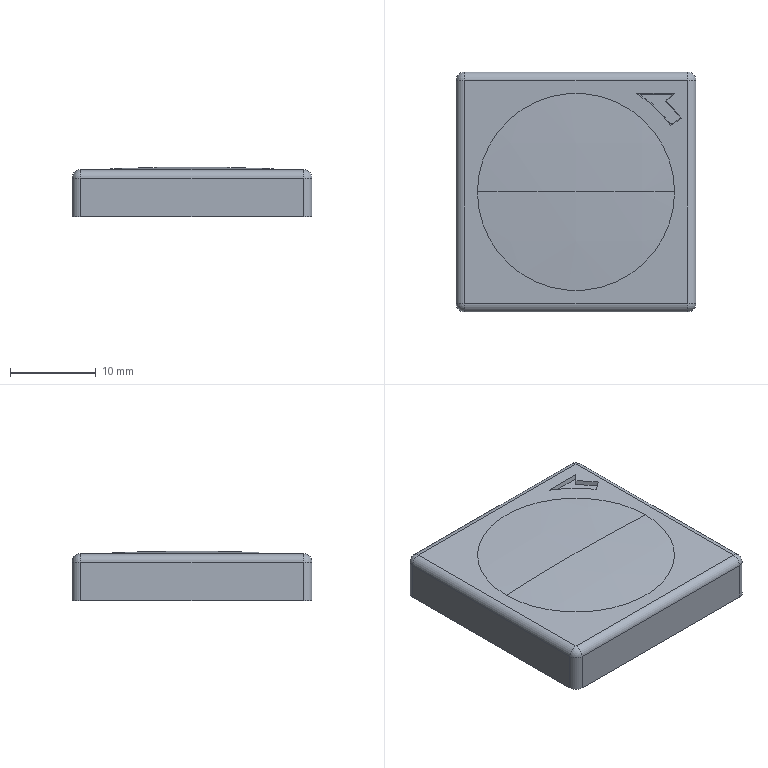Part | STEP file | AW30-03E_AW3020A Gauge_30-E | 1 solid | 26 faces | box 28 x 28 x 5.8 mm | volume 4343 mm3 | plane 10 | cylinder 8 | sphere 6 | cone 2 | commonest cylinder face diameters 2 x8
STEP:
#1=CARTESIAN_POINT('',(11.5,0.,0.));
#2=VERTEX_POINT('',#1);
#3=CARTESIAN_POINT('',(-11.5,0.,0.));
#4=VERTEX_POINT('',#3);
#5=CARTESIAN_POINT('',(0.,0.,0.));
#6=DIRECTION('',(0.,0.,1.));
#7=DIRECTION('',(-1.,0.,0.));
#8=AXIS2_PLACEMENT_3D('',#5,#6,#7);
#9=CIRCLE('',#8,11.5);
#10=EDGE_CURVE('',#2,#4,#9,.T.);
#11=ORIENTED_EDGE('',*,*,#10,.T.);
#12=CARTESIAN_POINT('',(0.,0.,0.3));
#13=VERTEX_POINT('',#12);
#14=CARTESIAN_POINT('',(0.,0.,-220.267));
#15=DIRECTION('',(0.,1.,0.));
#16=DIRECTION('',(-1.,0.,0.));
#17=AXIS2_PLACEMENT_3D('',#14,#15,#16);
#18=CIRCLE('',#17,220.567);
#19=EDGE_CURVE('',#4,#13,#18,.T.);
#20=ORIENTED_EDGE('',*,*,#19,.T.);
#21=CARTESIAN_POINT('',(0.,0.,-220.267));
#22=DIRECTION('',(0.,-1.,0.));
#23=DIRECTION('',(0.,0.,-1.));
#24=AXIS2_PLACEMENT_3D('',#21,#22,#23);
#25=CIRCLE('',#24,220.567);
#26=EDGE_CURVE('',#2,#13,#25,.T.);
#27=ORIENTED_EDGE('',*,*,#26,.F.);
#28=EDGE_LOOP('',(#11,#20,#27));
#29=FACE_OUTER_BOUND('',#28,.T.);
#30=CARTESIAN_POINT('',(0.,0.,-220.267));
#31=DIRECTION('',(0.,1.,0.));
#32=DIRECTION('',(1.,0.,0.));
#33=AXIS2_PLACEMENT_3D('',#30,#31,#32);
#34=SPHERICAL_SURFACE('',#33,220.567);
#35=ADVANCED_FACE('',(#29),#34,.T.);
#36=CARTESIAN_POINT('',(11.059,7.743,0.));
#37=VERTEX_POINT('',#36);
#38=CARTESIAN_POINT('',(12.287,8.604,0.));
#39=VERTEX_POINT('',#38);
#40=CARTESIAN_POINT('',(12.287,8.604,0.));
#41=DIRECTION('',(0.8192,0.5736,0.));
#42=VECTOR('',#41,1000.);
#43=LINE('',#40,#42);
#44=EDGE_CURVE('',#37,#39,#43,.T.);
#45=ORIENTED_EDGE('',*,*,#44,.F.);
#46=CARTESIAN_POINT('',(7.071,11.5,0.));
#47=VERTEX_POINT('',#46);
#48=CARTESIAN_POINT('',(0.,0.,0.));
#49=DIRECTION('',(0.,0.,-1.));
#50=DIRECTION('',(-1.,0.,0.));
#51=AXIS2_PLACEMENT_3D('',#48,#49,#50);
#52=CIRCLE('',#51,13.5);
#53=EDGE_CURVE('',#47,#37,#52,.T.);
#54=ORIENTED_EDGE('',*,*,#53,.F.);
#55=CARTESIAN_POINT('',(11.5,11.5,0.));
#56=VERTEX_POINT('',#55);
#57=CARTESIAN_POINT('',(7.071,11.5,0.));
#58=DIRECTION('',(-1.,0.,0.));
#59=VECTOR('',#58,1000.);
#60=LINE('',#57,#59);
#61=EDGE_CURVE('',#56,#47,#60,.T.);
#62=ORIENTED_EDGE('',*,*,#61,.F.);
#63=CARTESIAN_POINT('',(10.607,10.607,0.));
#64=VERTEX_POINT('',#63);
#65=CARTESIAN_POINT('',(11.5,11.5,0.));
#66=DIRECTION('',(0.7071,0.7071,0.));
#67=VECTOR('',#66,1000.);
#68=LINE('',#65,#67);
#69=EDGE_CURVE('',#64,#56,#68,.T.);
#70=ORIENTED_EDGE('',*,*,#69,.F.);
#71=CARTESIAN_POINT('',(0.,0.,0.));
#72=DIRECTION('',(0.,0.,1.));
#73=DIRECTION('',(-1.,0.,0.));
#74=AXIS2_PLACEMENT_3D('',#71,#72,#73);
#75=CIRCLE('',#74,15.);
#76=EDGE_CURVE('',#39,#64,#75,.T.);
#77=ORIENTED_EDGE('',*,*,#76,.F.);
#78=EDGE_LOOP('',(#45,#54,#62,#70,#77));
#79=FACE_BOUND('',#78,.T.);
#80=CARTESIAN_POINT('',(13.,-13.,0.));
#81=VERTEX_POINT('',#80);
#82=CARTESIAN_POINT('',(13.,13.,0.));
#83=VERTEX_POINT('',#82);
#84=CARTESIAN_POINT('',(13.,14.,0.));
#85=DIRECTION('',(0.,1.,0.));
#86=VECTOR('',#85,1000.);
#87=LINE('',#84,#86);
#88=EDGE_CURVE('',#81,#83,#87,.T.);
#89=ORIENTED_EDGE('',*,*,#88,.T.);
#90=CARTESIAN_POINT('',(-13.,13.,0.));
#91=VERTEX_POINT('',#90);
#92=CARTESIAN_POINT('',(-14.,13.,0.));
#93=DIRECTION('',(-1.,0.,0.));
#94=VECTOR('',#93,1000.);
#95=LINE('',#92,#94);
#96=EDGE_CURVE('',#83,#91,#95,.T.);
#97=ORIENTED_EDGE('',*,*,#96,.T.);
#98=CARTESIAN_POINT('',(-13.,-13.,0.));
#99=VERTEX_POINT('',#98);
#100=CARTESIAN_POINT('',(-13.,-14.,0.));
#101=DIRECTION('',(0.,-1.,0.));
#102=VECTOR('',#101,1000.);
#103=LINE('',#100,#102);
#104=EDGE_CURVE('',#91,#99,#103,.T.);
#105=ORIENTED_EDGE('',*,*,#104,.T.);
#106=CARTESIAN_POINT('',(14.,-13.,0.));
#107=DIRECTION('',(1.,0.,0.));
#108=VECTOR('',#107,1000.);
#109=LINE('',#106,#108);
#110=EDGE_CURVE('',#99,#81,#109,.T.);
#111=ORIENTED_EDGE('',*,*,#110,.T.);
#112=EDGE_LOOP('',(#89,#97,#105,#111));
#113=FACE_OUTER_BOUND('',#112,.T.);
#114=ORIENTED_EDGE('',*,*,#10,.F.);
#115=CARTESIAN_POINT('',(0.,0.,0.));
#116=DIRECTION('',(0.,0.,1.));
#117=DIRECTION('',(-1.,0.,0.));
#118=AXIS2_PLACEMENT_3D('',#115,#116,#117);
#119=CIRCLE('',#118,11.5);
#120=EDGE_CURVE('',#4,#2,#119,.T.);
#121=ORIENTED_EDGE('',*,*,#120,.F.);
#122=EDGE_LOOP('',(#114,#121));
#123=FACE_BOUND('',#122,.T.);
#124=CARTESIAN_POINT('',(14.,-14.,0.));
#125=DIRECTION('',(0.,0.,-1.));
#126=DIRECTION('',(-1.,0.,0.));
#127=AXIS2_PLACEMENT_3D('',#124,#125,#126);
#128=PLANE('',#127);
#129=ADVANCED_FACE('',(#79,#113,#123),#128,.F.);
#130=CARTESIAN_POINT('',(14.,-13.,-5.5));
#131=VERTEX_POINT('',#130);
#132=CARTESIAN_POINT('',(14.,13.,-5.5));
#133=VERTEX_POINT('',#132);
#134=CARTESIAN_POINT('',(14.,14.,-5.5));
#135=DIRECTION('',(0.,1.,0.));
#136=VECTOR('',#135,1000.);
#137=LINE('',#134,#136);
#138=EDGE_CURVE('',#131,#133,#137,.T.);
#139=ORIENTED_EDGE('',*,*,#138,.T.);
#140=CARTESIAN_POINT('',(14.,13.,-1.));
#141=VERTEX_POINT('',#140);
#142=CARTESIAN_POINT('',(14.,13.,-5.5));
#143=DIRECTION('',(0.,0.,1.));
#144=VECTOR('',#143,1000.);
#145=LINE('',#142,#144);
#146=EDGE_CURVE('',#133,#141,#145,.T.);
#147=ORIENTED_EDGE('',*,*,#146,.T.);
#148=CARTESIAN_POINT('',(14.,-13.,-1.));
#149=VERTEX_POINT('',#148);
#150=CARTESIAN_POINT('',(14.,-14.,-1.));
#151=DIRECTION('',(0.,-1.,0.));
#152=VECTOR('',#151,1000.);
#153=LINE('',#150,#152);
#154=EDGE_CURVE('',#141,#149,#153,.T.);
#155=ORIENTED_EDGE('',*,*,#154,.T.);
#156=CARTESIAN_POINT('',(14.,-13.,-5.5));
#157=DIRECTION('',(0.,0.,-1.));
#158=VECTOR('',#157,1000.);
#159=LINE('',#156,#158);
#160=EDGE_CURVE('',#149,#131,#159,.T.);
#161=ORIENTED_EDGE('',*,*,#160,.T.);
#162=EDGE_LOOP('',(#139,#147,#155,#161));
#163=FACE_OUTER_BOUND('',#162,.T.);
#164=CARTESIAN_POINT('',(14.,14.,-5.5));
#165=DIRECTION('',(1.,0.,0.));
#166=DIRECTION('',(0.,1.,0.));
#167=AXIS2_PLACEMENT_3D('',#164,#165,#166);
#168=PLANE('',#167);
#169=ADVANCED_FACE('',(#163),#168,.T.);
#170=CARTESIAN_POINT('',(-13.,-14.,-5.5));
#171=VERTEX_POINT('',#170);
#172=CARTESIAN_POINT('',(13.,-14.,-5.5));
#173=VERTEX_POINT('',#172);
#174=CARTESIAN_POINT('',(14.,-14.,-5.5));
#175=DIRECTION('',(1.,0.,0.));
#176=VECTOR('',#175,1000.);
#177=LINE('',#174,#176);
#178=EDGE_CURVE('',#171,#173,#177,.T.);
#179=ORIENTED_EDGE('',*,*,#178,.T.);
#180=CARTESIAN_POINT('',(13.,-14.,-1.));
#181=VERTEX_POINT('',#180);
#182=CARTESIAN_POINT('',(13.,-14.,-5.5));
#183=DIRECTION('',(0.,0.,1.));
#184=VECTOR('',#183,1000.);
#185=LINE('',#182,#184);
#186=EDGE_CURVE('',#173,#181,#185,.T.);
#187=ORIENTED_EDGE('',*,*,#186,.T.);
#188=CARTESIAN_POINT('',(-13.,-14.,-1.));
#189=VERTEX_POINT('',#188);
#190=CARTESIAN_POINT('',(-14.,-14.,-1.));
#191=DIRECTION('',(-1.,0.,0.));
#192=VECTOR('',#191,1000.);
#193=LINE('',#190,#192);
#194=EDGE_CURVE('',#181,#189,#193,.T.);
#195=ORIENTED_EDGE('',*,*,#194,.T.);
#196=CARTESIAN_POINT('',(-13.,-14.,-5.5));
#197=DIRECTION('',(0.,0.,-1.));
#198=VECTOR('',#197,1000.);
#199=LINE('',#196,#198);
#200=EDGE_CURVE('',#189,#171,#199,.T.);
#201=ORIENTED_EDGE('',*,*,#200,.T.);
#202=EDGE_LOOP('',(#179,#187,#195,#201));
#203=FACE_OUTER_BOUND('',#202,.T.);
#204=CARTESIAN_POINT('',(14.,-14.,-5.5));
#205=DIRECTION('',(0.,-1.,0.));
#206=DIRECTION('',(1.,0.,0.));
#207=AXIS2_PLACEMENT_3D('',#204,#205,#206);
#208=PLANE('',#207);
#209=ADVANCED_FACE('',(#203),#208,.T.);
#210=CARTESIAN_POINT('',(-14.,13.,-5.5));
#211=VERTEX_POINT('',#210);
#212=CARTESIAN_POINT('',(-14.,-13.,-5.5));
#213=VERTEX_POINT('',#212);
#214=CARTESIAN_POINT('',(-14.,14.,-5.5));
#215=DIRECTION('',(0.,-1.,0.));
#216=VECTOR('',#215,1000.);
#217=LINE('',#214,#216);
#218=EDGE_CURVE('',#211,#213,#217,.T.);
#219=ORIENTED_EDGE('',*,*,#218,.T.);
#220=CARTESIAN_POINT('',(-14.,-13.,-1.));
#221=VERTEX_POINT('',#220);
#222=CARTESIAN_POINT('',(-14.,-13.,-5.5));
#223=DIRECTION('',(0.,0.,1.));
#224=VECTOR('',#223,1000.);
#225=LINE('',#222,#224);
#226=EDGE_CURVE('',#213,#221,#225,.T.);
#227=ORIENTED_EDGE('',*,*,#226,.T.);
#228=CARTESIAN_POINT('',(-14.,13.,-1.));
#229=VERTEX_POINT('',#228);
#230=CARTESIAN_POINT('',(-14.,14.,-1.));
#231=DIRECTION('',(0.,1.,0.));
#232=VECTOR('',#231,1000.);
#233=LINE('',#230,#232);
#234=EDGE_CURVE('',#221,#229,#233,.T.);
#235=ORIENTED_EDGE('',*,*,#234,.T.);
#236=CARTESIAN_POINT('',(-14.,13.,-5.5));
#237=DIRECTION('',(0.,0.,-1.));
#238=VECTOR('',#237,1000.);
#239=LINE('',#236,#238);
#240=EDGE_CURVE('',#229,#211,#239,.T.);
#241=ORIENTED_EDGE('',*,*,#240,.T.);
#242=EDGE_LOOP('',(#219,#227,#235,#241));
#243=FACE_OUTER_BOUND('',#242,.T.);
#244=CARTESIAN_POINT('',(-14.,14.,-5.5));
#245=DIRECTION('',(-1.,0.,0.));
#246=DIRECTION('',(0.,-1.,0.));
#247=AXIS2_PLACEMENT_3D('',#244,#245,#246);
#248=PLANE('',#247);
#249=ADVANCED_FACE('',(#243),#248,.T.);
#250=CARTESIAN_POINT('',(-13.,14.,-1.));
#251=VERTEX_POINT('',#250);
#252=CARTESIAN_POINT('',(13.,14.,-1.));
#253=VERTEX_POINT('',#252);
#254=CARTESIAN_POINT('',(14.,14.,-1.));
#255=DIRECTION('',(1.,0.,0.));
#256=VECTOR('',#255,1000.);
#257=LINE('',#254,#256);
#258=EDGE_CURVE('',#251,#253,#257,.T.);
#259=ORIENTED_EDGE('',*,*,#258,.T.);
#260=CARTESIAN_POINT('',(13.,14.,-5.5));
#261=VERTEX_POINT('',#260);
#262=CARTESIAN_POINT('',(13.,14.,-5.5));
#263=DIRECTION('',(0.,0.,-1.));
#264=VECTOR('',#263,1000.);
#265=LINE('',#262,#264);
#266=EDGE_CURVE('',#253,#261,#265,.T.);
#267=ORIENTED_EDGE('',*,*,#266,.T.);
#268=CARTESIAN_POINT('',(-13.,14.,-5.5));
#269=VERTEX_POINT('',#268);
#270=CARTESIAN_POINT('',(14.,14.,-5.5));
#271=DIRECTION('',(-1.,0.,0.));
#272=VECTOR('',#271,1000.);
#273=LINE('',#270,#272);
#274=EDGE_CURVE('',#261,#269,#273,.T.);
#275=ORIENTED_EDGE('',*,*,#274,.T.);
#276=CARTESIAN_POINT('',(-13.,14.,-5.5));
#277=DIRECTION('',(0.,0.,1.));
#278=VECTOR('',#277,1000.);
#279=LINE('',#276,#278);
#280=EDGE_CURVE('',#269,#251,#279,.T.);
#281=ORIENTED_EDGE('',*,*,#280,.T.);
#282=EDGE_LOOP('',(#259,#267,#275,#281));
#283=FACE_OUTER_BOUND('',#282,.T.);
#284=CARTESIAN_POINT('',(14.,14.,-5.5));
#285=DIRECTION('',(0.,1.,0.));
#286=DIRECTION('',(-1.,0.,0.));
#287=AXIS2_PLACEMENT_3D('',#284,#285,#286);
#288=PLANE('',#287);
#289=ADVANCED_FACE('',(#283),#288,.T.);
#290=ORIENTED_EDGE('',*,*,#274,.F.);
#291=CARTESIAN_POINT('',(13.,13.,-5.5));
#292=DIRECTION('',(0.,0.,-1.));
#293=DIRECTION('',(-1.,0.,0.));
#294=AXIS2_PLACEMENT_3D('',#291,#292,#293);
#295=CIRCLE('',#294,1.);
#296=EDGE_CURVE('',#261,#133,#295,.T.);
#297=ORIENTED_EDGE('',*,*,#296,.T.);
#298=ORIENTED_EDGE('',*,*,#138,.F.);
#299=CARTESIAN_POINT('',(13.,-13.,-5.5));
#300=DIRECTION('',(0.,0.,-1.));
#301=DIRECTION('',(-1.,0.,0.));
#302=AXIS2_PLACEMENT_3D('',#299,#300,#301);
#303=CIRCLE('',#302,1.);
#304=EDGE_CURVE('',#131,#173,#303,.T.);
#305=ORIENTED_EDGE('',*,*,#304,.T.);
#306=ORIENTED_EDGE('',*,*,#178,.F.);
#307=CARTESIAN_POINT('',(-13.,-13.,-5.5));
#308=DIRECTION('',(0.,0.,-1.));
#309=DIRECTION('',(-1.,0.,0.));
#310=AXIS2_PLACEMENT_3D('',#307,#308,#309);
#311=CIRCLE('',#310,1.);
#312=EDGE_CURVE('',#171,#213,#311,.T.);
#313=ORIENTED_EDGE('',*,*,#312,.T.);
#314=ORIENTED_EDGE('',*,*,#218,.F.);
#315=CARTESIAN_POINT('',(-13.,13.,-5.5));
#316=DIRECTION('',(0.,0.,-1.));
#317=DIRECTION('',(-1.,0.,0.));
#318=AXIS2_PLACEMENT_3D('',#315,#316,#317);
#319=CIRCLE('',#318,1.);
#320=EDGE_CURVE('',#211,#269,#319,.T.);
#321=ORIENTED_EDGE('',*,*,#320,.T.);
#322=EDGE_LOOP('',(#290,#297,#298,#305,#306,#313,#314,#321));
#323=FACE_OUTER_BOUND('',#322,.T.);
#324=CARTESIAN_POINT('',(14.,-14.,-5.5));
#325=DIRECTION('',(0.,0.,-1.));
#326=DIRECTION('',(-1.,0.,0.));
#327=AXIS2_PLACEMENT_3D('',#324,#325,#326);
#328=PLANE('',#327);
#329=ADVANCED_FACE('',(#323),#328,.T.);
#330=ORIENTED_EDGE('',*,*,#19,.F.);
#331=ORIENTED_EDGE('',*,*,#120,.T.);
#332=ORIENTED_EDGE('',*,*,#26,.T.);
#333=EDGE_LOOP('',(#330,#331,#332));
#334=FACE_OUTER_BOUND('',#333,.T.);
#335=CARTESIAN_POINT('',(0.,0.,-220.267));
#336=DIRECTION('',(0.,1.,0.));
#337=DIRECTION('',(1.,0.,0.));
#338=AXIS2_PLACEMENT_3D('',#335,#336,#337);
#339=SPHERICAL_SURFACE('',#338,220.567);
#340=ADVANCED_FACE('',(#334),#339,.T.);
#341=ORIENTED_EDGE('',*,*,#304,.F.);
#342=ORIENTED_EDGE('',*,*,#160,.F.);
#343=CARTESIAN_POINT('',(13.,-13.,-1.));
#344=DIRECTION('',(0.,0.,1.));
#345=DIRECTION('',(1.,0.,0.));
#346=AXIS2_PLACEMENT_3D('',#343,#344,#345);
#347=CIRCLE('',#346,1.);
#348=EDGE_CURVE('',#181,#149,#347,.T.);
#349=ORIENTED_EDGE('',*,*,#348,.F.);
#350=ORIENTED_EDGE('',*,*,#186,.F.);
#351=EDGE_LOOP('',(#341,#342,#349,#350));
#352=FACE_OUTER_BOUND('',#351,.T.);
#353=CARTESIAN_POINT('',(13.,-13.,-5.5));
#354=DIRECTION('',(0.,0.,1.));
#355=DIRECTION('',(1.,0.,0.));
#356=AXIS2_PLACEMENT_3D('',#353,#354,#355);
#357=CYLINDRICAL_SURFACE('',#356,1.);
#358=ADVANCED_FACE('',(#352),#357,.T.);
#359=CARTESIAN_POINT('',(-13.,-13.,-1.));
#360=DIRECTION('',(-1.,0.,0.));
#361=DIRECTION('',(0.,0.,1.));
#362=AXIS2_PLACEMENT_3D('',#359,#360,#361);
#363=CIRCLE('',#362,1.);
#364=EDGE_CURVE('',#189,#99,#363,.T.);
#365=ORIENTED_EDGE('',*,*,#364,.F.);
#366=ORIENTED_EDGE('',*,*,#194,.F.);
#367=CARTESIAN_POINT('',(13.,-13.,-1.));
#368=DIRECTION('',(1.,0.,0.));
#369=DIRECTION('',(0.,0.,-1.));
#370=AXIS2_PLACEMENT_3D('',#367,#368,#369);
#371=CIRCLE('',#370,1.);
#372=EDGE_CURVE('',#81,#181,#371,.T.);
#373=ORIENTED_EDGE('',*,*,#372,.F.);
#374=ORIENTED_EDGE('',*,*,#110,.F.);
#375=EDGE_LOOP('',(#365,#366,#373,#374));
#376=FACE_OUTER_BOUND('',#375,.T.);
#377=CARTESIAN_POINT('',(14.,-13.,-1.));
#378=DIRECTION('',(-1.,0.,0.));
#379=DIRECTION('',(0.,-1.,0.));
#380=AXIS2_PLACEMENT_3D('',#377,#378,#379);
#381=CYLINDRICAL_SURFACE('',#380,1.);
#382=ADVANCED_FACE('',(#376),#381,.T.);
#383=ORIENTED_EDGE('',*,*,#312,.F.);
#384=ORIENTED_EDGE('',*,*,#200,.F.);
#385=CARTESIAN_POINT('',(-13.,-13.,-1.));
#386=DIRECTION('',(0.,0.,1.));
#387=DIRECTION('',(1.,0.,0.));
#388=AXIS2_PLACEMENT_3D('',#385,#386,#387);
#389=CIRCLE('',#388,1.);
#390=EDGE_CURVE('',#221,#189,#389,.T.);
#391=ORIENTED_EDGE('',*,*,#390,.F.);
#392=ORIENTED_EDGE('',*,*,#226,.F.);
#393=EDGE_LOOP('',(#383,#384,#391,#392));
#394=FACE_OUTER_BOUND('',#393,.T.);
#395=CARTESIAN_POINT('',(-13.,-13.,-5.5));
#396=DIRECTION('',(0.,0.,1.));
#397=DIRECTION('',(1.,0.,0.));
#398=AXIS2_PLACEMENT_3D('',#395,#396,#397);
#399=CYLINDRICAL_SURFACE('',#398,1.);
#400=ADVANCED_FACE('',(#394),#399,.T.);
#401=ORIENTED_EDGE('',*,*,#372,.T.);
#402=ORIENTED_EDGE('',*,*,#348,.T.);
#403=CARTESIAN_POINT('',(13.,-13.,-1.));
#404=DIRECTION('',(0.,1.,0.));
#405=DIRECTION('',(0.,0.,-1.));
#406=AXIS2_PLACEMENT_3D('',#403,#404,#405);
#407=CIRCLE('',#406,1.);
#408=EDGE_CURVE('',#81,#149,#407,.T.);
#409=ORIENTED_EDGE('',*,*,#408,.F.);
#410=EDGE_LOOP('',(#401,#402,#409));
#411=FACE_OUTER_BOUND('',#410,.T.);
#412=CARTESIAN_POINT('',(13.,-13.,-1.));
#413=DIRECTION('',(0.,1.,0.));
#414=DIRECTION('',(1.,0.,0.));
#415=AXIS2_PLACEMENT_3D('',#412,#413,#414);
#416=SPHERICAL_SURFACE('',#415,1.);
#417=ADVANCED_FACE('',(#411),#416,.T.);
#418=ORIENTED_EDGE('',*,*,#390,.T.);
#419=ORIENTED_EDGE('',*,*,#364,.T.);
#420=CARTESIAN_POINT('',(-13.,-13.,-1.));
#421=DIRECTION('',(0.,1.,0.));
#422=DIRECTION('',(0.,0.,-1.));
#423=AXIS2_PLACEMENT_3D('',#420,#421,#422);
#424=CIRCLE('',#423,1.);
#425=EDGE_CURVE('',#221,#99,#424,.T.);
#426=ORIENTED_EDGE('',*,*,#425,.F.);
#427=EDGE_LOOP('',(#418,#419,#426));
#428=FACE_OUTER_BOUND('',#427,.T.);
#429=CARTESIAN_POINT('',(-13.,-13.,-1.));
#430=DIRECTION('',(0.,1.,0.));
#431=DIRECTION('',(1.,0.,0.));
#432=AXIS2_PLACEMENT_3D('',#429,#430,#431);
#433=SPHERICAL_SURFACE('',#432,1.);
#434=ADVANCED_FACE('',(#428),#433,.T.);
#435=ORIENTED_EDGE('',*,*,#296,.F.);
#436=ORIENTED_EDGE('',*,*,#266,.F.);
#437=CARTESIAN_POINT('',(13.,13.,-1.));
#438=DIRECTION('',(0.,0.,1.));
#439=DIRECTION('',(1.,0.,0.));
#440=AXIS2_PLACEMENT_3D('',#437,#438,#439);
#441=CIRCLE('',#440,1.);
#442=EDGE_CURVE('',#141,#253,#441,.T.);
#443=ORIENTED_EDGE('',*,*,#442,.F.);
#444=ORIENTED_EDGE('',*,*,#146,.F.);
#445=EDGE_LOOP('',(#435,#436,#443,#444));
#446=FACE_OUTER_BOUND('',#445,.T.);
#447=CARTESIAN_POINT('',(13.,13.,-5.5));
#448=DIRECTION('',(0.,0.,1.));
#449=DIRECTION('',(1.,0.,0.));
#450=AXIS2_PLACEMENT_3D('',#447,#448,#449);
#451=CYLINDRICAL_SURFACE('',#450,1.);
#452=ADVANCED_FACE('',(#446),#451,.T.);
#453=ORIENTED_EDGE('',*,*,#408,.T.);
#454=ORIENTED_EDGE('',*,*,#154,.F.);
#455=CARTESIAN_POINT('',(13.,13.,-1.));
#456=DIRECTION('',(0.,1.,0.));
#457=DIRECTION('',(0.,0.,1.));
#458=AXIS2_PLACEMENT_3D('',#455,#456,#457);
#459=CIRCLE('',#458,1.);
#460=EDGE_CURVE('',#83,#141,#459,.T.);
#461=ORIENTED_EDGE('',*,*,#460,.F.);
#462=ORIENTED_EDGE('',*,*,#88,.F.);
#463=EDGE_LOOP('',(#453,#454,#461,#462));
#464=FACE_OUTER_BOUND('',#463,.T.);
#465=CARTESIAN_POINT('',(13.,-14.,-1.));
#466=DIRECTION('',(0.,-1.,0.));
#467=DIRECTION('',(1.,0.,0.));
#468=AXIS2_PLACEMENT_3D('',#465,#466,#467);
#469=CYLINDRICAL_SURFACE('',#468,1.);
#470=ADVANCED_FACE('',(#464),#469,.T.);
#471=ORIENTED_EDGE('',*,*,#425,.T.);
#472=ORIENTED_EDGE('',*,*,#104,.F.);
#473=CARTESIAN_POINT('',(-13.,13.,-1.));
#474=DIRECTION('',(0.,1.,0.));
#475=DIRECTION('',(0.,0.,1.));
#476=AXIS2_PLACEMENT_3D('',#473,#474,#475);
#477=CIRCLE('',#476,1.);
#478=EDGE_CURVE('',#229,#91,#477,.T.);
#479=ORIENTED_EDGE('',*,*,#478,.F.);
#480=ORIENTED_EDGE('',*,*,#234,.F.);
#481=EDGE_LOOP('',(#471,#472,#479,#480));
#482=FACE_OUTER_BOUND('',#481,.T.);
#483=CARTESIAN_POINT('',(-13.,-14.,-1.));
#484=DIRECTION('',(0.,1.,0.));
#485=DIRECTION('',(-1.,0.,0.));
#486=AXIS2_PLACEMENT_3D('',#483,#484,#485);
#487=CYLINDRICAL_SURFACE('',#486,1.);
#488=ADVANCED_FACE('',(#482),#487,.T.);
#489=ORIENTED_EDGE('',*,*,#320,.F.);
#490=ORIENTED_EDGE('',*,*,#240,.F.);
#491=CARTESIAN_POINT('',(-13.,13.,-1.));
#492=DIRECTION('',(0.,0.,1.));
#493=DIRECTION('',(1.,0.,0.));
#494=AXIS2_PLACEMENT_3D('',#491,#492,#493);
#495=CIRCLE('',#494,1.);
#496=EDGE_CURVE('',#251,#229,#495,.T.);
#497=ORIENTED_EDGE('',*,*,#496,.F.);
#498=ORIENTED_EDGE('',*,*,#280,.F.);
#499=EDGE_LOOP('',(#489,#490,#497,#498));
#500=FACE_OUTER_BOUND('',#499,.T.);
#501=CARTESIAN_POINT('',(-13.,13.,-5.5));
#502=DIRECTION('',(0.,0.,1.));
#503=DIRECTION('',(1.,0.,0.));
#504=AXIS2_PLACEMENT_3D('',#501,#502,#503);
#505=CYLINDRICAL_SURFACE('',#504,1.);
#506=ADVANCED_FACE('',(#500),#505,.T.);
#507=ORIENTED_EDGE('',*,*,#460,.T.);
#508=ORIENTED_EDGE('',*,*,#442,.T.);
#509=CARTESIAN_POINT('',(13.,13.,-1.));
#510=DIRECTION('',(-1.,0.,0.));
#511=DIRECTION('',(0.,0.,-1.));
#512=AXIS2_PLACEMENT_3D('',#509,#510,#511);
#513=CIRCLE('',#512,1.);
#514=EDGE_CURVE('',#83,#253,#513,.T.);
#515=ORIENTED_EDGE('',*,*,#514,.F.);
#516=EDGE_LOOP('',(#507,#508,#515));
#517=FACE_OUTER_BOUND('',#516,.T.);
#518=CARTESIAN_POINT('',(13.,13.,-1.));
#519=DIRECTION('',(0.,1.,0.));
#520=DIRECTION('',(1.,0.,0.));
#521=AXIS2_PLACEMENT_3D('',#518,#519,#520);
#522=SPHERICAL_SURFACE('',#521,1.);
#523=ADVANCED_FACE('',(#517),#522,.T.);
#524=ORIENTED_EDGE('',*,*,#496,.T.);
#525=ORIENTED_EDGE('',*,*,#478,.T.);
#526=CARTESIAN_POINT('',(-13.,13.,-1.));
#527=DIRECTION('',(1.,0.,0.));
#528=DIRECTION('',(0.,-1.,0.));
#529=AXIS2_PLACEMENT_3D('',#526,#527,#528);
#530=CIRCLE('',#529,1.);
#531=EDGE_CURVE('',#251,#91,#530,.T.);
#532=ORIENTED_EDGE('',*,*,#531,.F.);
#533=EDGE_LOOP('',(#524,#525,#532));
#534=FACE_OUTER_BOUND('',#533,.T.);
#535=CARTESIAN_POINT('',(-13.,13.,-1.));
#536=DIRECTION('',(0.,1.,0.));
#537=DIRECTION('',(1.,0.,0.));
#538=AXIS2_PLACEMENT_3D('',#535,#536,#537);
#539=SPHERICAL_SURFACE('',#538,1.);
#540=ADVANCED_FACE('',(#534),#539,.T.);
#541=ORIENTED_EDGE('',*,*,#514,.T.);
#542=ORIENTED_EDGE('',*,*,#258,.F.);
#543=ORIENTED_EDGE('',*,*,#531,.T.);
#544=ORIENTED_EDGE('',*,*,#96,.F.);
#545=EDGE_LOOP('',(#541,#542,#543,#544));
#546=FACE_OUTER_BOUND('',#545,.T.);
#547=CARTESIAN_POINT('',(14.,13.,-1.));
#548=DIRECTION('',(1.,0.,0.));
#549=DIRECTION('',(0.,1.,0.));
#550=AXIS2_PLACEMENT_3D('',#547,#548,#549);
#551=CYLINDRICAL_SURFACE('',#550,1.);
#552=ADVANCED_FACE('',(#546),#551,.T.);
#553=ORIENTED_EDGE('',*,*,#53,.T.);
#554=CARTESIAN_POINT('',(11.08,7.866,-0.5));
#555=VERTEX_POINT('',#554);
#556=CARTESIAN_POINT('',(11.08,7.866,-0.5));
#557=CARTESIAN_POINT('',(11.073,7.825,-0.3333));
#558=CARTESIAN_POINT('',(11.066,7.784,-0.1667));
#559=CARTESIAN_POINT('',(11.059,7.743,0.));
#560=B_SPLINE_CURVE_WITH_KNOTS('',3,(#556,#557,#558,#559),.UNSPECIFIED.,.F.,.F.,(4,4),(0.,0.0005153),.UNSPECIFIED.);
#561=EDGE_CURVE('',#555,#37,#560,.T.);
#562=ORIENTED_EDGE('',*,*,#561,.F.);
#563=CARTESIAN_POINT('',(7.376,11.412,-0.5));
#564=VERTEX_POINT('',#563);
#565=CARTESIAN_POINT('',(0.,0.,-0.5));
#566=DIRECTION('',(0.,0.,-1.));
#567=DIRECTION('',(-1.,0.,0.));
#568=AXIS2_PLACEMENT_3D('',#565,#566,#567);
#569=CIRCLE('',#568,13.588);
#570=EDGE_CURVE('',#564,#555,#569,.T.);
#571=ORIENTED_EDGE('',*,*,#570,.F.);
#572=CARTESIAN_POINT('',(7.376,11.412,-0.5));
#573=CARTESIAN_POINT('',(7.276,11.441,-0.3324));
#574=CARTESIAN_POINT('',(7.174,11.471,-0.1657));
#575=CARTESIAN_POINT('',(7.071,11.5,0.));
#576=B_SPLINE_CURVE_WITH_KNOTS('',3,(#572,#573,#574,#575),.UNSPECIFIED.,.F.,.F.,(4,4),(0.,0.0005923),.UNSPECIFIED.);
#577=EDGE_CURVE('',#564,#47,#576,.T.);
#578=ORIENTED_EDGE('',*,*,#577,.T.);
#579=EDGE_LOOP('',(#553,#562,#571,#578));
#580=FACE_OUTER_BOUND('',#579,.T.);
#581=CARTESIAN_POINT('',(0.,0.,0.));
#582=DIRECTION('',(0.,0.,-1.));
#583=DIRECTION('',(-1.,0.,0.));
#584=AXIS2_PLACEMENT_3D('',#581,#582,#583);
#585=CONICAL_SURFACE('',#584,13.5,0.1745);
#586=ADVANCED_FACE('',(#580),#585,.T.);
#587=ORIENTED_EDGE('',*,*,#61,.T.);
#588=ORIENTED_EDGE('',*,*,#577,.F.);
#589=CARTESIAN_POINT('',(11.287,11.412,-0.5));
#590=VERTEX_POINT('',#589);
#591=CARTESIAN_POINT('',(7.071,11.412,-0.5));
#592=DIRECTION('',(-1.,0.,0.));
#593=VECTOR('',#592,1000.);
#594=LINE('',#591,#593);
#595=EDGE_CURVE('',#590,#564,#594,.T.);
#596=ORIENTED_EDGE('',*,*,#595,.F.);
#597=CARTESIAN_POINT('',(11.5,11.5,0.));
#598=DIRECTION('',(0.3866,0.1601,0.9082));
#599=VECTOR('',#598,1000.);
#600=LINE('',#597,#599);
#601=EDGE_CURVE('',#590,#56,#600,.T.);
#602=ORIENTED_EDGE('',*,*,#601,.T.);
#603=EDGE_LOOP('',(#587,#588,#596,#602));
#604=FACE_OUTER_BOUND('',#603,.T.);
#605=CARTESIAN_POINT('',(7.071,11.5,0.));
#606=DIRECTION('',(0.,0.9848,-0.1736));
#607=DIRECTION('',(0.,0.1736,0.9848));
#608=AXIS2_PLACEMENT_3D('',#605,#606,#607);
#609=PLANE('',#608);
#610=ADVANCED_FACE('',(#604),#609,.F.);
#611=ORIENTED_EDGE('',*,*,#69,.T.);
#612=ORIENTED_EDGE('',*,*,#601,.F.);
#613=CARTESIAN_POINT('',(10.482,10.606,-0.5));
#614=VERTEX_POINT('',#613);
#615=CARTESIAN_POINT('',(11.438,11.562,-0.5));
#616=DIRECTION('',(0.7071,0.7071,0.));
#617=VECTOR('',#616,1000.);
#618=LINE('',#615,#617);
#619=EDGE_CURVE('',#614,#590,#618,.T.);
#620=ORIENTED_EDGE('',*,*,#619,.F.);
#621=CARTESIAN_POINT('',(10.482,10.606,-0.5));
#622=CARTESIAN_POINT('',(10.523,10.607,-0.3333));
#623=CARTESIAN_POINT('',(10.565,10.607,-0.1667));
#624=CARTESIAN_POINT('',(10.607,10.607,0.));
#625=B_SPLINE_CURVE_WITH_KNOTS('',3,(#621,#622,#623,#624),.UNSPECIFIED.,.F.,.F.,(4,4),(0.,0.0005154),.UNSPECIFIED.);
#626=EDGE_CURVE('',#614,#64,#625,.T.);
#627=ORIENTED_EDGE('',*,*,#626,.T.);
#628=EDGE_LOOP('',(#611,#612,#620,#627));
#629=FACE_OUTER_BOUND('',#628,.T.);
#630=CARTESIAN_POINT('',(11.5,11.5,0.));
#631=DIRECTION('',(0.6964,-0.6964,-0.1736));
#632=DIRECTION('',(0.7071,0.7071,0.));
#633=AXIS2_PLACEMENT_3D('',#630,#631,#632);
#634=PLANE('',#633);
#635=ADVANCED_FACE('',(#629),#634,.F.);
#636=ORIENTED_EDGE('',*,*,#76,.T.);
#637=ORIENTED_EDGE('',*,*,#626,.F.);
#638=CARTESIAN_POINT('',(12.164,8.625,-0.5));
#639=VERTEX_POINT('',#638);
#640=CARTESIAN_POINT('',(0.,0.,-0.5));
#641=DIRECTION('',(0.,0.,1.));
#642=DIRECTION('',(-1.,0.,0.));
#643=AXIS2_PLACEMENT_3D('',#640,#641,#642);
#644=CIRCLE('',#643,14.912);
#645=EDGE_CURVE('',#639,#614,#644,.T.);
#646=ORIENTED_EDGE('',*,*,#645,.F.);
#647=CARTESIAN_POINT('',(12.164,8.625,-0.5));
#648=CARTESIAN_POINT('',(12.205,8.618,-0.3333));
#649=CARTESIAN_POINT('',(12.246,8.611,-0.1667));
#650=CARTESIAN_POINT('',(12.287,8.604,0.));
#651=B_SPLINE_CURVE_WITH_KNOTS('',3,(#647,#648,#649,#650),.UNSPECIFIED.,.F.,.F.,(4,4),(0.,0.0005154),.UNSPECIFIED.);
#652=EDGE_CURVE('',#639,#39,#651,.T.);
#653=ORIENTED_EDGE('',*,*,#652,.T.);
#654=EDGE_LOOP('',(#636,#637,#646,#653));
#655=FACE_OUTER_BOUND('',#654,.T.);
#656=CARTESIAN_POINT('',(0.,0.,0.));
#657=DIRECTION('',(0.,0.,1.));
#658=DIRECTION('',(-1.,0.,0.));
#659=AXIS2_PLACEMENT_3D('',#656,#657,#658);
#660=CONICAL_SURFACE('',#659,15.,0.1745);
#661=ADVANCED_FACE('',(#655),#660,.F.);
#662=ORIENTED_EDGE('',*,*,#44,.T.);
#663=ORIENTED_EDGE('',*,*,#652,.F.);
#664=CARTESIAN_POINT('',(12.237,8.676,-0.5));
#665=DIRECTION('',(0.8192,0.5736,0.));
#666=VECTOR('',#665,1000.);
#667=LINE('',#664,#666);
#668=EDGE_CURVE('',#555,#639,#667,.T.);
#669=ORIENTED_EDGE('',*,*,#668,.F.);
#670=ORIENTED_EDGE('',*,*,#561,.T.);
#671=EDGE_LOOP('',(#662,#663,#669,#670));
#672=FACE_OUTER_BOUND('',#671,.T.);
#673=CARTESIAN_POINT('',(12.287,8.604,0.));
#674=DIRECTION('',(0.5649,-0.8067,-0.1736));
#675=DIRECTION('',(0.8192,0.5736,0.));
#676=AXIS2_PLACEMENT_3D('',#673,#674,#675);
#677=PLANE('',#676);
#678=ADVANCED_FACE('',(#672),#677,.F.);
#679=ORIENTED_EDGE('',*,*,#570,.T.);
#680=ORIENTED_EDGE('',*,*,#668,.T.);
#681=ORIENTED_EDGE('',*,*,#645,.T.);
#682=ORIENTED_EDGE('',*,*,#619,.T.);
#683=ORIENTED_EDGE('',*,*,#595,.T.);
#684=EDGE_LOOP('',(#679,#680,#681,#682,#683));
#685=FACE_OUTER_BOUND('',#684,.T.);
#686=CARTESIAN_POINT('',(0.,0.,-0.5));
#687=DIRECTION('',(0.,0.,-1.));
#688=DIRECTION('',(-1.,0.,0.));
#689=AXIS2_PLACEMENT_3D('',#686,#687,#688);
#690=PLANE('',#689);
#691=ADVANCED_FACE('',(#685),#690,.F.);
#692=CLOSED_SHELL('',(#35,#129,#169,#209,#249,#289,#329,#340,#358,#382,#400,#417,#434,#452,#470,#488,#506,#523,#540,#552,#586,#610,#635,#661,#678,#691));
#693=MANIFOLD_SOLID_BREP('',#692);
#694=CARTESIAN_POINT('',(0.,0.,0.));
#695=DIRECTION('',(0.,0.,1.));
#696=DIRECTION('',(1.,0.,0.));
#697=AXIS2_PLACEMENT_3D('',#694,#695,#696);
#698=(LENGTH_UNIT()NAMED_UNIT(*)SI_UNIT(.MILLI.,.METRE.));
#699=UNCERTAINTY_MEASURE_WITH_UNIT(LENGTH_MEASURE(0.00001),#698,'','');
#700=(NAMED_UNIT(*)PLANE_ANGLE_UNIT()SI_UNIT($,.RADIAN.));
#701=(NAMED_UNIT(*)SI_UNIT($,.STERADIAN.)SOLID_ANGLE_UNIT());
#702=(GEOMETRIC_REPRESENTATION_CONTEXT(3)GLOBAL_UNCERTAINTY_ASSIGNED_CONTEXT((#699))GLOBAL_UNIT_ASSIGNED_CONTEXT((#698,#700,#701))REPRESENTATION_CONTEXT('',''));
#703=ADVANCED_BREP_SHAPE_REPRESENTATION('',(#693,#697),#702);